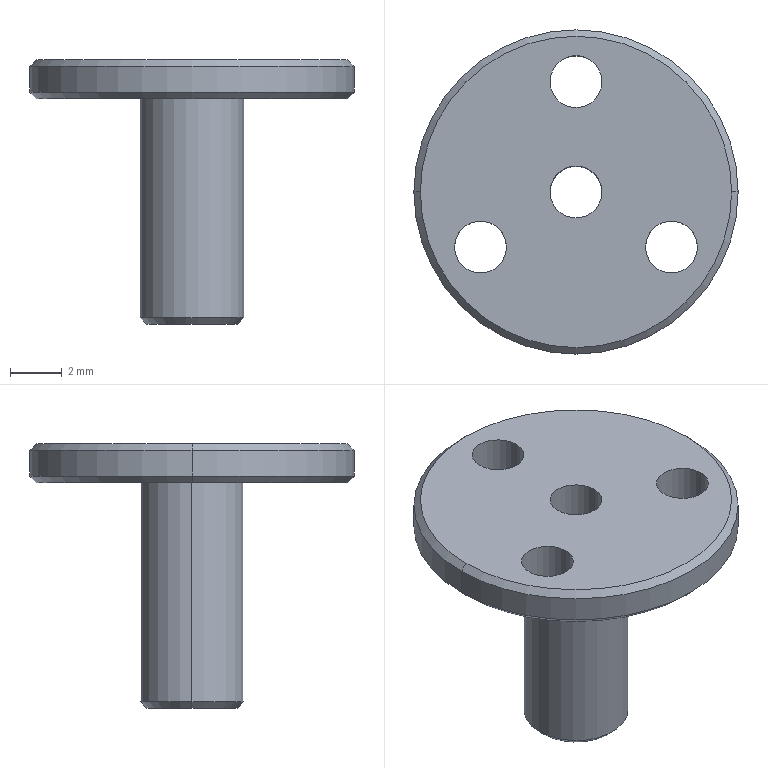Part | NX | features BREP 1 | 1 solid | 21 faces | box 12.5 x 12.5 x 10.2 mm | volume 244.426 mm3 | cylinder 12 | cone 6 | plane 3 | commonest cylinder face diameters 2 x8 4 x2 12.5 x2
STEP:
#1=CARTESIAN_POINT('',(30.496,239.617,-8.7));
#2=VERTEX_POINT('',#1);
#3=CARTESIAN_POINT('',(33.996,239.617,-8.7));
#4=VERTEX_POINT('',#3);
#5=CARTESIAN_POINT('',(32.246,239.617,-8.7));
#6=DIRECTION('',(0.,0.,-1.));
#7=DIRECTION('',(-1.,0.,0.));
#8=AXIS2_PLACEMENT_3D('',#5,#6,#7);
#9=CIRCLE('',#8,1.75);
#10=EDGE_CURVE('',#2,#4,#9,.T.);
#11=ORIENTED_EDGE('',*,*,#10,.F.);
#12=CARTESIAN_POINT('',(30.246,239.617,-8.45));
#13=VERTEX_POINT('',#12);
#14=CARTESIAN_POINT('',(30.496,239.617,-8.7));
#15=DIRECTION('',(-0.7071,0.,0.7071));
#16=VECTOR('',#15,1000.);
#17=LINE('',#14,#16);
#18=EDGE_CURVE('',#2,#13,#17,.T.);
#19=ORIENTED_EDGE('',*,*,#18,.T.);
#20=CARTESIAN_POINT('',(34.246,239.617,-8.45));
#21=VERTEX_POINT('',#20);
#22=CARTESIAN_POINT('',(32.246,239.617,-8.45));
#23=DIRECTION('',(0.,0.,1.));
#24=DIRECTION('',(-1.,0.,0.));
#25=AXIS2_PLACEMENT_3D('',#22,#23,#24);
#26=CIRCLE('',#25,2.);
#27=EDGE_CURVE('',#21,#13,#26,.T.);
#28=ORIENTED_EDGE('',*,*,#27,.F.);
#29=CARTESIAN_POINT('',(33.996,239.617,-8.7));
#30=DIRECTION('',(0.7071,0.,0.7071));
#31=VECTOR('',#30,1000.);
#32=LINE('',#29,#31);
#33=EDGE_CURVE('',#4,#21,#32,.T.);
#34=ORIENTED_EDGE('',*,*,#33,.F.);
#35=EDGE_LOOP('',(#11,#19,#28,#34));
#36=FACE_BOUND('',#35,.T.);
#37=CARTESIAN_POINT('',(32.246,239.617,-8.7));
#38=DIRECTION('',(0.,0.,1.));
#39=DIRECTION('',(-1.,0.,0.));
#40=AXIS2_PLACEMENT_3D('',#37,#38,#39);
#41=CONICAL_SURFACE('',#40,1.75,0.7854);
#42=ADVANCED_FACE('',(#36),#41,.T.);
#43=CARTESIAN_POINT('',(38.246,239.617,1.5));
#44=VERTEX_POINT('',#43);
#45=CARTESIAN_POINT('',(26.246,239.617,1.5));
#46=VERTEX_POINT('',#45);
#47=CARTESIAN_POINT('',(32.246,239.617,1.5));
#48=DIRECTION('',(0.,0.,1.));
#49=DIRECTION('',(1.,0.,0.));
#50=AXIS2_PLACEMENT_3D('',#47,#48,#49);
#51=CIRCLE('',#50,6.);
#52=EDGE_CURVE('',#44,#46,#51,.T.);
#53=ORIENTED_EDGE('',*,*,#52,.F.);
#54=CARTESIAN_POINT('',(38.496,239.617,1.25));
#55=VERTEX_POINT('',#54);
#56=CARTESIAN_POINT('',(38.246,239.617,1.5));
#57=DIRECTION('',(0.7071,0.,-0.7071));
#58=VECTOR('',#57,1000.);
#59=LINE('',#56,#58);
#60=EDGE_CURVE('',#55,#44,#59,.F.);
#61=ORIENTED_EDGE('',*,*,#60,.F.);
#62=CARTESIAN_POINT('',(25.996,239.617,1.25));
#63=VERTEX_POINT('',#62);
#64=CARTESIAN_POINT('',(32.246,239.617,1.25));
#65=DIRECTION('',(0.,0.,-1.));
#66=DIRECTION('',(1.,0.,0.));
#67=AXIS2_PLACEMENT_3D('',#64,#65,#66);
#68=CIRCLE('',#67,6.25);
#69=EDGE_CURVE('',#63,#55,#68,.T.);
#70=ORIENTED_EDGE('',*,*,#69,.F.);
#71=CARTESIAN_POINT('',(26.246,239.617,1.5));
#72=DIRECTION('',(-0.7071,0.,-0.7071));
#73=VECTOR('',#72,1000.);
#74=LINE('',#71,#73);
#75=EDGE_CURVE('',#63,#46,#74,.F.);
#76=ORIENTED_EDGE('',*,*,#75,.T.);
#77=EDGE_LOOP('',(#53,#61,#70,#76));
#78=FACE_BOUND('',#77,.T.);
#79=CARTESIAN_POINT('',(32.246,239.617,1.5));
#80=DIRECTION('',(0.,0.,-1.));
#81=DIRECTION('',(1.,0.,0.));
#82=AXIS2_PLACEMENT_3D('',#79,#80,#81);
#83=CONICAL_SURFACE('',#82,6.,0.7854);
#84=ADVANCED_FACE('',(#78),#83,.T.);
#85=CARTESIAN_POINT('',(26.246,239.617,0.));
#86=VERTEX_POINT('',#85);
#87=CARTESIAN_POINT('',(38.246,239.617,0.));
#88=VERTEX_POINT('',#87);
#89=CARTESIAN_POINT('',(32.246,239.617,0.));
#90=DIRECTION('',(0.,0.,-1.));
#91=DIRECTION('',(1.,0.,0.));
#92=AXIS2_PLACEMENT_3D('',#89,#90,#91);
#93=CIRCLE('',#92,6.);
#94=EDGE_CURVE('',#86,#88,#93,.T.);
#95=ORIENTED_EDGE('',*,*,#94,.F.);
#96=CARTESIAN_POINT('',(25.996,239.617,0.25));
#97=VERTEX_POINT('',#96);
#98=CARTESIAN_POINT('',(25.996,239.617,0.25));
#99=DIRECTION('',(-0.7071,0.,0.7071));
#100=VECTOR('',#99,1000.);
#101=LINE('',#98,#100);
#102=EDGE_CURVE('',#86,#97,#101,.T.);
#103=ORIENTED_EDGE('',*,*,#102,.T.);
#104=CARTESIAN_POINT('',(38.496,239.617,0.25));
#105=VERTEX_POINT('',#104);
#106=CARTESIAN_POINT('',(32.246,239.617,0.25));
#107=DIRECTION('',(0.,0.,1.));
#108=DIRECTION('',(1.,0.,0.));
#109=AXIS2_PLACEMENT_3D('',#106,#107,#108);
#110=CIRCLE('',#109,6.25);
#111=EDGE_CURVE('',#105,#97,#110,.T.);
#112=ORIENTED_EDGE('',*,*,#111,.F.);
#113=CARTESIAN_POINT('',(38.496,239.617,0.25));
#114=DIRECTION('',(0.7071,0.,0.7071));
#115=VECTOR('',#114,1000.);
#116=LINE('',#113,#115);
#117=EDGE_CURVE('',#88,#105,#116,.T.);
#118=ORIENTED_EDGE('',*,*,#117,.F.);
#119=EDGE_LOOP('',(#95,#103,#112,#118));
#120=FACE_BOUND('',#119,.T.);
#121=CARTESIAN_POINT('',(32.246,239.617,0.25));
#122=DIRECTION('',(0.,0.,1.));
#123=DIRECTION('',(-1.,0.,0.));
#124=AXIS2_PLACEMENT_3D('',#121,#122,#123);
#125=CONICAL_SURFACE('',#124,6.25,0.7854);
#126=ADVANCED_FACE('',(#120),#125,.T.);
#127=CARTESIAN_POINT('',(31.246,239.617,1.5));
#128=VERTEX_POINT('',#127);
#129=CARTESIAN_POINT('',(33.246,239.617,1.5));
#130=VERTEX_POINT('',#129);
#131=CARTESIAN_POINT('',(32.246,239.617,1.5));
#132=DIRECTION('',(0.,0.,1.));
#133=DIRECTION('',(1.,0.,0.));
#134=AXIS2_PLACEMENT_3D('',#131,#132,#133);
#135=CIRCLE('',#134,1.);
#136=EDGE_CURVE('',#128,#130,#135,.T.);
#137=ORIENTED_EDGE('',*,*,#136,.T.);
#138=CARTESIAN_POINT('',(33.246,239.617,-8.7));
#139=VERTEX_POINT('',#138);
#140=CARTESIAN_POINT('',(33.246,239.617,-2.7));
#141=DIRECTION('',(0.,0.,-1.));
#142=VECTOR('',#141,1000.);
#143=LINE('',#140,#142);
#144=EDGE_CURVE('',#139,#130,#143,.F.);
#145=ORIENTED_EDGE('',*,*,#144,.F.);
#146=CARTESIAN_POINT('',(31.246,239.617,-8.7));
#147=VERTEX_POINT('',#146);
#148=CARTESIAN_POINT('',(32.246,239.617,-8.7));
#149=DIRECTION('',(0.,0.,-1.));
#150=DIRECTION('',(-1.,0.,0.));
#151=AXIS2_PLACEMENT_3D('',#148,#149,#150);
#152=CIRCLE('',#151,1.);
#153=EDGE_CURVE('',#139,#147,#152,.T.);
#154=ORIENTED_EDGE('',*,*,#153,.T.);
#155=CARTESIAN_POINT('',(31.246,239.617,-2.7));
#156=DIRECTION('',(0.,0.,-1.));
#157=VECTOR('',#156,1000.);
#158=LINE('',#155,#157);
#159=EDGE_CURVE('',#147,#128,#158,.F.);
#160=ORIENTED_EDGE('',*,*,#159,.T.);
#161=EDGE_LOOP('',(#137,#145,#154,#160));
#162=FACE_BOUND('',#161,.T.);
#163=CARTESIAN_POINT('',(32.246,239.617,-2.7));
#164=DIRECTION('',(0.,0.,-1.));
#165=DIRECTION('',(1.,0.,0.));
#166=AXIS2_PLACEMENT_3D('',#163,#164,#165);
#167=CYLINDRICAL_SURFACE('',#166,1.);
#168=ADVANCED_FACE('',(#162),#167,.F.);
#169=ORIENTED_EDGE('',*,*,#27,.T.);
#170=CARTESIAN_POINT('',(30.246,239.617,0.));
#171=VERTEX_POINT('',#170);
#172=CARTESIAN_POINT('',(30.246,239.617,-14.357));
#173=DIRECTION('',(0.,0.,1.));
#174=VECTOR('',#173,1000.);
#175=LINE('',#172,#174);
#176=EDGE_CURVE('',#13,#171,#175,.T.);
#177=ORIENTED_EDGE('',*,*,#176,.T.);
#178=CARTESIAN_POINT('',(34.246,239.617,0.));
#179=VERTEX_POINT('',#178);
#180=CARTESIAN_POINT('',(32.246,239.617,0.));
#181=DIRECTION('',(0.,0.,-1.));
#182=DIRECTION('',(1.,0.,0.));
#183=AXIS2_PLACEMENT_3D('',#180,#181,#182);
#184=CIRCLE('',#183,2.);
#185=EDGE_CURVE('',#171,#179,#184,.T.);
#186=ORIENTED_EDGE('',*,*,#185,.T.);
#187=CARTESIAN_POINT('',(34.246,239.617,-14.357));
#188=DIRECTION('',(0.,0.,1.));
#189=VECTOR('',#188,1000.);
#190=LINE('',#187,#189);
#191=EDGE_CURVE('',#21,#179,#190,.T.);
#192=ORIENTED_EDGE('',*,*,#191,.F.);
#193=EDGE_LOOP('',(#169,#177,#186,#192));
#194=FACE_BOUND('',#193,.T.);
#195=CARTESIAN_POINT('',(32.246,239.617,-14.357));
#196=DIRECTION('',(0.,0.,1.));
#197=DIRECTION('',(-1.,0.,0.));
#198=AXIS2_PLACEMENT_3D('',#195,#196,#197);
#199=CYLINDRICAL_SURFACE('',#198,2.);
#200=ADVANCED_FACE('',(#194),#199,.T.);
#201=CARTESIAN_POINT('',(27.566,237.492,1.5));
#202=VERTEX_POINT('',#201);
#203=CARTESIAN_POINT('',(29.566,237.492,1.5));
#204=VERTEX_POINT('',#203);
#205=CARTESIAN_POINT('',(28.566,237.492,1.5));
#206=DIRECTION('',(0.,0.,1.));
#207=DIRECTION('',(1.,0.,0.));
#208=AXIS2_PLACEMENT_3D('',#205,#206,#207);
#209=CIRCLE('',#208,1.);
#210=EDGE_CURVE('',#202,#204,#209,.T.);
#211=ORIENTED_EDGE('',*,*,#210,.T.);
#212=CARTESIAN_POINT('',(29.566,237.492,0.));
#213=VERTEX_POINT('',#212);
#214=CARTESIAN_POINT('',(29.566,237.492,1.5));
#215=DIRECTION('',(0.,0.,-1.));
#216=VECTOR('',#215,1000.);
#217=LINE('',#214,#216);
#218=EDGE_CURVE('',#213,#204,#217,.F.);
#219=ORIENTED_EDGE('',*,*,#218,.F.);
#220=CARTESIAN_POINT('',(27.566,237.492,0.));
#221=VERTEX_POINT('',#220);
#222=CARTESIAN_POINT('',(28.566,237.492,0.));
#223=DIRECTION('',(0.,0.,1.));
#224=DIRECTION('',(1.,0.,0.));
#225=AXIS2_PLACEMENT_3D('',#222,#223,#224);
#226=CIRCLE('',#225,1.);
#227=EDGE_CURVE('',#221,#213,#226,.T.);
#228=ORIENTED_EDGE('',*,*,#227,.F.);
#229=CARTESIAN_POINT('',(27.566,237.492,1.5));
#230=DIRECTION('',(0.,0.,-1.));
#231=VECTOR('',#230,1000.);
#232=LINE('',#229,#231);
#233=EDGE_CURVE('',#221,#202,#232,.F.);
#234=ORIENTED_EDGE('',*,*,#233,.T.);
#235=EDGE_LOOP('',(#211,#219,#228,#234));
#236=FACE_BOUND('',#235,.T.);
#237=CARTESIAN_POINT('',(28.566,237.492,1.5));
#238=DIRECTION('',(0.,0.,-1.));
#239=DIRECTION('',(1.,0.,0.));
#240=AXIS2_PLACEMENT_3D('',#237,#238,#239);
#241=CYLINDRICAL_SURFACE('',#240,1.);
#242=ADVANCED_FACE('',(#236),#241,.F.);
#243=CARTESIAN_POINT('',(34.927,237.492,1.5));
#244=VERTEX_POINT('',#243);
#245=CARTESIAN_POINT('',(36.927,237.492,1.5));
#246=VERTEX_POINT('',#245);
#247=CARTESIAN_POINT('',(35.927,237.492,1.5));
#248=DIRECTION('',(0.,0.,1.));
#249=DIRECTION('',(1.,0.,0.));
#250=AXIS2_PLACEMENT_3D('',#247,#248,#249);
#251=CIRCLE('',#250,1.);
#252=EDGE_CURVE('',#244,#246,#251,.T.);
#253=ORIENTED_EDGE('',*,*,#252,.T.);
#254=CARTESIAN_POINT('',(36.927,237.492,0.));
#255=VERTEX_POINT('',#254);
#256=CARTESIAN_POINT('',(36.927,237.492,1.5));
#257=DIRECTION('',(0.,0.,-1.));
#258=VECTOR('',#257,1000.);
#259=LINE('',#256,#258);
#260=EDGE_CURVE('',#255,#246,#259,.F.);
#261=ORIENTED_EDGE('',*,*,#260,.F.);
#262=CARTESIAN_POINT('',(34.927,237.492,0.));
#263=VERTEX_POINT('',#262);
#264=CARTESIAN_POINT('',(35.927,237.492,0.));
#265=DIRECTION('',(0.,0.,1.));
#266=DIRECTION('',(1.,0.,0.));
#267=AXIS2_PLACEMENT_3D('',#264,#265,#266);
#268=CIRCLE('',#267,1.);
#269=EDGE_CURVE('',#263,#255,#268,.T.);
#270=ORIENTED_EDGE('',*,*,#269,.F.);
#271=CARTESIAN_POINT('',(34.927,237.492,1.5));
#272=DIRECTION('',(0.,0.,-1.));
#273=VECTOR('',#272,1000.);
#274=LINE('',#271,#273);
#275=EDGE_CURVE('',#263,#244,#274,.F.);
#276=ORIENTED_EDGE('',*,*,#275,.T.);
#277=EDGE_LOOP('',(#253,#261,#270,#276));
#278=FACE_BOUND('',#277,.T.);
#279=CARTESIAN_POINT('',(35.927,237.492,1.5));
#280=DIRECTION('',(0.,0.,-1.));
#281=DIRECTION('',(1.,0.,0.));
#282=AXIS2_PLACEMENT_3D('',#279,#280,#281);
#283=CYLINDRICAL_SURFACE('',#282,1.);
#284=ADVANCED_FACE('',(#278),#283,.F.);
#285=CARTESIAN_POINT('',(31.246,243.867,1.5));
#286=VERTEX_POINT('',#285);
#287=CARTESIAN_POINT('',(33.246,243.867,1.5));
#288=VERTEX_POINT('',#287);
#289=CARTESIAN_POINT('',(32.246,243.867,1.5));
#290=DIRECTION('',(0.,0.,1.));
#291=DIRECTION('',(1.,0.,0.));
#292=AXIS2_PLACEMENT_3D('',#289,#290,#291);
#293=CIRCLE('',#292,1.);
#294=EDGE_CURVE('',#286,#288,#293,.T.);
#295=ORIENTED_EDGE('',*,*,#294,.T.);
#296=CARTESIAN_POINT('',(33.246,243.867,0.));
#297=VERTEX_POINT('',#296);
#298=CARTESIAN_POINT('',(33.246,243.867,1.5));
#299=DIRECTION('',(0.,0.,-1.));
#300=VECTOR('',#299,1000.);
#301=LINE('',#298,#300);
#302=EDGE_CURVE('',#297,#288,#301,.F.);
#303=ORIENTED_EDGE('',*,*,#302,.F.);
#304=CARTESIAN_POINT('',(31.246,243.867,0.));
#305=VERTEX_POINT('',#304);
#306=CARTESIAN_POINT('',(32.246,243.867,0.));
#307=DIRECTION('',(0.,0.,1.));
#308=DIRECTION('',(1.,0.,0.));
#309=AXIS2_PLACEMENT_3D('',#306,#307,#308);
#310=CIRCLE('',#309,1.);
#311=EDGE_CURVE('',#305,#297,#310,.T.);
#312=ORIENTED_EDGE('',*,*,#311,.F.);
#313=CARTESIAN_POINT('',(31.246,243.867,1.5));
#314=DIRECTION('',(0.,0.,-1.));
#315=VECTOR('',#314,1000.);
#316=LINE('',#313,#315);
#317=EDGE_CURVE('',#305,#286,#316,.F.);
#318=ORIENTED_EDGE('',*,*,#317,.T.);
#319=EDGE_LOOP('',(#295,#303,#312,#318));
#320=FACE_BOUND('',#319,.T.);
#321=CARTESIAN_POINT('',(32.246,243.867,1.5));
#322=DIRECTION('',(0.,0.,-1.));
#323=DIRECTION('',(1.,0.,0.));
#324=AXIS2_PLACEMENT_3D('',#321,#322,#323);
#325=CYLINDRICAL_SURFACE('',#324,1.);
#326=ADVANCED_FACE('',(#320),#325,.F.);
#327=ORIENTED_EDGE('',*,*,#69,.T.);
#328=CARTESIAN_POINT('',(38.496,239.617,1.5));
#329=DIRECTION('',(0.,0.,-1.));
#330=VECTOR('',#329,1000.);
#331=LINE('',#328,#330);
#332=EDGE_CURVE('',#105,#55,#331,.F.);
#333=ORIENTED_EDGE('',*,*,#332,.F.);
#334=ORIENTED_EDGE('',*,*,#111,.T.);
#335=CARTESIAN_POINT('',(25.996,239.617,1.5));
#336=DIRECTION('',(0.,0.,-1.));
#337=VECTOR('',#336,1000.);
#338=LINE('',#335,#337);
#339=EDGE_CURVE('',#97,#63,#338,.F.);
#340=ORIENTED_EDGE('',*,*,#339,.T.);
#341=EDGE_LOOP('',(#327,#333,#334,#340));
#342=FACE_BOUND('',#341,.T.);
#343=CARTESIAN_POINT('',(32.246,239.617,1.5));
#344=DIRECTION('',(0.,0.,-1.));
#345=DIRECTION('',(1.,0.,0.));
#346=AXIS2_PLACEMENT_3D('',#343,#344,#345);
#347=CYLINDRICAL_SURFACE('',#346,6.25);
#348=ADVANCED_FACE('',(#342),#347,.T.);
#349=CARTESIAN_POINT('',(32.246,239.617,1.5));
#350=DIRECTION('',(0.,0.,1.));
#351=DIRECTION('',(1.,0.,0.));
#352=AXIS2_PLACEMENT_3D('',#349,#350,#351);
#353=CIRCLE('',#352,6.);
#354=EDGE_CURVE('',#46,#44,#353,.T.);
#355=ORIENTED_EDGE('',*,*,#354,.T.);
#356=ORIENTED_EDGE('',*,*,#52,.T.);
#357=EDGE_LOOP('',(#355,#356));
#358=FACE_BOUND('',#357,.T.);
#359=ORIENTED_EDGE('',*,*,#136,.F.);
#360=CARTESIAN_POINT('',(32.246,239.617,1.5));
#361=DIRECTION('',(0.,0.,1.));
#362=DIRECTION('',(1.,0.,0.));
#363=AXIS2_PLACEMENT_3D('',#360,#361,#362);
#364=CIRCLE('',#363,1.);
#365=EDGE_CURVE('',#130,#128,#364,.T.);
#366=ORIENTED_EDGE('',*,*,#365,.F.);
#367=EDGE_LOOP('',(#359,#366));
#368=FACE_BOUND('',#367,.T.);
#369=ORIENTED_EDGE('',*,*,#252,.F.);
#370=CARTESIAN_POINT('',(35.927,237.492,1.5));
#371=DIRECTION('',(0.,0.,1.));
#372=DIRECTION('',(1.,0.,0.));
#373=AXIS2_PLACEMENT_3D('',#370,#371,#372);
#374=CIRCLE('',#373,1.);
#375=EDGE_CURVE('',#246,#244,#374,.T.);
#376=ORIENTED_EDGE('',*,*,#375,.F.);
#377=EDGE_LOOP('',(#369,#376));
#378=FACE_BOUND('',#377,.T.);
#379=ORIENTED_EDGE('',*,*,#294,.F.);
#380=CARTESIAN_POINT('',(32.246,243.867,1.5));
#381=DIRECTION('',(0.,0.,1.));
#382=DIRECTION('',(1.,0.,0.));
#383=AXIS2_PLACEMENT_3D('',#380,#381,#382);
#384=CIRCLE('',#383,1.);
#385=EDGE_CURVE('',#288,#286,#384,.T.);
#386=ORIENTED_EDGE('',*,*,#385,.F.);
#387=EDGE_LOOP('',(#379,#386));
#388=FACE_BOUND('',#387,.T.);
#389=ORIENTED_EDGE('',*,*,#210,.F.);
#390=CARTESIAN_POINT('',(28.566,237.492,1.5));
#391=DIRECTION('',(0.,0.,1.));
#392=DIRECTION('',(1.,0.,0.));
#393=AXIS2_PLACEMENT_3D('',#390,#391,#392);
#394=CIRCLE('',#393,1.);
#395=EDGE_CURVE('',#204,#202,#394,.T.);
#396=ORIENTED_EDGE('',*,*,#395,.F.);
#397=EDGE_LOOP('',(#389,#396));
#398=FACE_BOUND('',#397,.T.);
#399=CARTESIAN_POINT('',(32.246,239.617,1.5));
#400=DIRECTION('',(0.,0.,1.));
#401=DIRECTION('',(-1.,0.,0.));
#402=AXIS2_PLACEMENT_3D('',#399,#400,#401);
#403=PLANE('',#402);
#404=ADVANCED_FACE('',(#358,#368,#378,#388,#398),#403,.T.);
#405=CARTESIAN_POINT('',(32.246,239.617,0.));
#406=DIRECTION('',(0.,0.,-1.));
#407=DIRECTION('',(1.,0.,0.));
#408=AXIS2_PLACEMENT_3D('',#405,#406,#407);
#409=CIRCLE('',#408,6.);
#410=EDGE_CURVE('',#88,#86,#409,.T.);
#411=ORIENTED_EDGE('',*,*,#410,.T.);
#412=ORIENTED_EDGE('',*,*,#94,.T.);
#413=EDGE_LOOP('',(#411,#412));
#414=FACE_BOUND('',#413,.T.);
#415=CARTESIAN_POINT('',(32.246,239.617,0.));
#416=DIRECTION('',(0.,0.,-1.));
#417=DIRECTION('',(1.,0.,0.));
#418=AXIS2_PLACEMENT_3D('',#415,#416,#417);
#419=CIRCLE('',#418,2.);
#420=EDGE_CURVE('',#179,#171,#419,.T.);
#421=ORIENTED_EDGE('',*,*,#420,.F.);
#422=ORIENTED_EDGE('',*,*,#185,.F.);
#423=EDGE_LOOP('',(#421,#422));
#424=FACE_BOUND('',#423,.T.);
#425=ORIENTED_EDGE('',*,*,#311,.T.);
#426=CARTESIAN_POINT('',(32.246,243.867,0.));
#427=DIRECTION('',(0.,0.,1.));
#428=DIRECTION('',(1.,0.,0.));
#429=AXIS2_PLACEMENT_3D('',#426,#427,#428);
#430=CIRCLE('',#429,1.);
#431=EDGE_CURVE('',#297,#305,#430,.T.);
#432=ORIENTED_EDGE('',*,*,#431,.T.);
#433=EDGE_LOOP('',(#425,#432));
#434=FACE_BOUND('',#433,.T.);
#435=ORIENTED_EDGE('',*,*,#269,.T.);
#436=CARTESIAN_POINT('',(35.927,237.492,0.));
#437=DIRECTION('',(0.,0.,1.));
#438=DIRECTION('',(1.,0.,0.));
#439=AXIS2_PLACEMENT_3D('',#436,#437,#438);
#440=CIRCLE('',#439,1.);
#441=EDGE_CURVE('',#255,#263,#440,.T.);
#442=ORIENTED_EDGE('',*,*,#441,.T.);
#443=EDGE_LOOP('',(#435,#442));
#444=FACE_BOUND('',#443,.T.);
#445=ORIENTED_EDGE('',*,*,#227,.T.);
#446=CARTESIAN_POINT('',(28.566,237.492,0.));
#447=DIRECTION('',(0.,0.,1.));
#448=DIRECTION('',(1.,0.,0.));
#449=AXIS2_PLACEMENT_3D('',#446,#447,#448);
#450=CIRCLE('',#449,1.);
#451=EDGE_CURVE('',#213,#221,#450,.T.);
#452=ORIENTED_EDGE('',*,*,#451,.T.);
#453=EDGE_LOOP('',(#445,#452));
#454=FACE_BOUND('',#453,.T.);
#455=CARTESIAN_POINT('',(32.246,239.617,0.));
#456=DIRECTION('',(0.,0.,1.));
#457=DIRECTION('',(-1.,0.,0.));
#458=AXIS2_PLACEMENT_3D('',#455,#456,#457);
#459=PLANE('',#458);
#460=ADVANCED_FACE('',(#414,#424,#434,#444,#454),#459,.F.);
#461=ORIENTED_EDGE('',*,*,#332,.T.);
#462=CARTESIAN_POINT('',(32.246,239.617,1.25));
#463=DIRECTION('',(0.,0.,-1.));
#464=DIRECTION('',(1.,0.,0.));
#465=AXIS2_PLACEMENT_3D('',#462,#463,#464);
#466=CIRCLE('',#465,6.25);
#467=EDGE_CURVE('',#55,#63,#466,.T.);
#468=ORIENTED_EDGE('',*,*,#467,.T.);
#469=ORIENTED_EDGE('',*,*,#339,.F.);
#470=CARTESIAN_POINT('',(32.246,239.617,0.25));
#471=DIRECTION('',(0.,0.,1.));
#472=DIRECTION('',(1.,0.,0.));
#473=AXIS2_PLACEMENT_3D('',#470,#471,#472);
#474=CIRCLE('',#473,6.25);
#475=EDGE_CURVE('',#97,#105,#474,.T.);
#476=ORIENTED_EDGE('',*,*,#475,.T.);
#477=EDGE_LOOP('',(#461,#468,#469,#476));
#478=FACE_BOUND('',#477,.T.);
#479=CARTESIAN_POINT('',(32.246,239.617,1.5));
#480=DIRECTION('',(0.,0.,-1.));
#481=DIRECTION('',(1.,0.,0.));
#482=AXIS2_PLACEMENT_3D('',#479,#480,#481);
#483=CYLINDRICAL_SURFACE('',#482,6.25);
#484=ADVANCED_FACE('',(#478),#483,.T.);
#485=ORIENTED_EDGE('',*,*,#302,.T.);
#486=ORIENTED_EDGE('',*,*,#385,.T.);
#487=ORIENTED_EDGE('',*,*,#317,.F.);
#488=ORIENTED_EDGE('',*,*,#431,.F.);
#489=EDGE_LOOP('',(#485,#486,#487,#488));
#490=FACE_BOUND('',#489,.T.);
#491=CARTESIAN_POINT('',(32.246,243.867,1.5));
#492=DIRECTION('',(0.,0.,-1.));
#493=DIRECTION('',(1.,0.,0.));
#494=AXIS2_PLACEMENT_3D('',#491,#492,#493);
#495=CYLINDRICAL_SURFACE('',#494,1.);
#496=ADVANCED_FACE('',(#490),#495,.F.);
#497=ORIENTED_EDGE('',*,*,#260,.T.);
#498=ORIENTED_EDGE('',*,*,#375,.T.);
#499=ORIENTED_EDGE('',*,*,#275,.F.);
#500=ORIENTED_EDGE('',*,*,#441,.F.);
#501=EDGE_LOOP('',(#497,#498,#499,#500));
#502=FACE_BOUND('',#501,.T.);
#503=CARTESIAN_POINT('',(35.927,237.492,1.5));
#504=DIRECTION('',(0.,0.,-1.));
#505=DIRECTION('',(1.,0.,0.));
#506=AXIS2_PLACEMENT_3D('',#503,#504,#505);
#507=CYLINDRICAL_SURFACE('',#506,1.);
#508=ADVANCED_FACE('',(#502),#507,.F.);
#509=ORIENTED_EDGE('',*,*,#218,.T.);
#510=ORIENTED_EDGE('',*,*,#395,.T.);
#511=ORIENTED_EDGE('',*,*,#233,.F.);
#512=ORIENTED_EDGE('',*,*,#451,.F.);
#513=EDGE_LOOP('',(#509,#510,#511,#512));
#514=FACE_BOUND('',#513,.T.);
#515=CARTESIAN_POINT('',(28.566,237.492,1.5));
#516=DIRECTION('',(0.,0.,-1.));
#517=DIRECTION('',(1.,0.,0.));
#518=AXIS2_PLACEMENT_3D('',#515,#516,#517);
#519=CYLINDRICAL_SURFACE('',#518,1.);
#520=ADVANCED_FACE('',(#514),#519,.F.);
#521=ORIENTED_EDGE('',*,*,#176,.F.);
#522=CARTESIAN_POINT('',(32.246,239.617,-8.45));
#523=DIRECTION('',(0.,0.,1.));
#524=DIRECTION('',(-1.,0.,0.));
#525=AXIS2_PLACEMENT_3D('',#522,#523,#524);
#526=CIRCLE('',#525,2.);
#527=EDGE_CURVE('',#13,#21,#526,.T.);
#528=ORIENTED_EDGE('',*,*,#527,.T.);
#529=ORIENTED_EDGE('',*,*,#191,.T.);
#530=ORIENTED_EDGE('',*,*,#420,.T.);
#531=EDGE_LOOP('',(#521,#528,#529,#530));
#532=FACE_BOUND('',#531,.T.);
#533=CARTESIAN_POINT('',(32.246,239.617,-14.357));
#534=DIRECTION('',(0.,0.,1.));
#535=DIRECTION('',(-1.,0.,0.));
#536=AXIS2_PLACEMENT_3D('',#533,#534,#535);
#537=CYLINDRICAL_SURFACE('',#536,2.);
#538=ADVANCED_FACE('',(#532),#537,.T.);
#539=CARTESIAN_POINT('',(32.246,239.617,-8.7));
#540=DIRECTION('',(0.,0.,-1.));
#541=DIRECTION('',(-1.,0.,0.));
#542=AXIS2_PLACEMENT_3D('',#539,#540,#541);
#543=CIRCLE('',#542,1.75);
#544=EDGE_CURVE('',#4,#2,#543,.T.);
#545=ORIENTED_EDGE('',*,*,#544,.T.);
#546=ORIENTED_EDGE('',*,*,#10,.T.);
#547=EDGE_LOOP('',(#545,#546));
#548=FACE_BOUND('',#547,.T.);
#549=CARTESIAN_POINT('',(32.246,239.617,-8.7));
#550=DIRECTION('',(0.,0.,-1.));
#551=DIRECTION('',(-1.,0.,0.));
#552=AXIS2_PLACEMENT_3D('',#549,#550,#551);
#553=CIRCLE('',#552,1.);
#554=EDGE_CURVE('',#147,#139,#553,.T.);
#555=ORIENTED_EDGE('',*,*,#554,.F.);
#556=ORIENTED_EDGE('',*,*,#153,.F.);
#557=EDGE_LOOP('',(#555,#556));
#558=FACE_BOUND('',#557,.T.);
#559=CARTESIAN_POINT('',(29.103,240.218,-8.7));
#560=DIRECTION('',(0.,0.,-1.));
#561=DIRECTION('',(0.,1.,0.));
#562=AXIS2_PLACEMENT_3D('',#559,#560,#561);
#563=PLANE('',#562);
#564=ADVANCED_FACE('',(#548,#558),#563,.T.);
#565=ORIENTED_EDGE('',*,*,#144,.T.);
#566=ORIENTED_EDGE('',*,*,#365,.T.);
#567=ORIENTED_EDGE('',*,*,#159,.F.);
#568=ORIENTED_EDGE('',*,*,#554,.T.);
#569=EDGE_LOOP('',(#565,#566,#567,#568));
#570=FACE_BOUND('',#569,.T.);
#571=CARTESIAN_POINT('',(32.246,239.617,-2.7));
#572=DIRECTION('',(0.,0.,-1.));
#573=DIRECTION('',(1.,0.,0.));
#574=AXIS2_PLACEMENT_3D('',#571,#572,#573);
#575=CYLINDRICAL_SURFACE('',#574,1.);
#576=ADVANCED_FACE('',(#570),#575,.F.);
#577=ORIENTED_EDGE('',*,*,#102,.F.);
#578=ORIENTED_EDGE('',*,*,#410,.F.);
#579=ORIENTED_EDGE('',*,*,#117,.T.);
#580=ORIENTED_EDGE('',*,*,#475,.F.);
#581=EDGE_LOOP('',(#577,#578,#579,#580));
#582=FACE_BOUND('',#581,.T.);
#583=CARTESIAN_POINT('',(32.246,239.617,0.25));
#584=DIRECTION('',(0.,0.,1.));
#585=DIRECTION('',(-1.,0.,0.));
#586=AXIS2_PLACEMENT_3D('',#583,#584,#585);
#587=CONICAL_SURFACE('',#586,6.25,0.7854);
#588=ADVANCED_FACE('',(#582),#587,.T.);
#589=ORIENTED_EDGE('',*,*,#60,.T.);
#590=ORIENTED_EDGE('',*,*,#354,.F.);
#591=ORIENTED_EDGE('',*,*,#75,.F.);
#592=ORIENTED_EDGE('',*,*,#467,.F.);
#593=EDGE_LOOP('',(#589,#590,#591,#592));
#594=FACE_BOUND('',#593,.T.);
#595=CARTESIAN_POINT('',(32.246,239.617,1.5));
#596=DIRECTION('',(0.,0.,-1.));
#597=DIRECTION('',(1.,0.,0.));
#598=AXIS2_PLACEMENT_3D('',#595,#596,#597);
#599=CONICAL_SURFACE('',#598,6.,0.7854);
#600=ADVANCED_FACE('',(#594),#599,.T.);
#601=ORIENTED_EDGE('',*,*,#18,.F.);
#602=ORIENTED_EDGE('',*,*,#544,.F.);
#603=ORIENTED_EDGE('',*,*,#33,.T.);
#604=ORIENTED_EDGE('',*,*,#527,.F.);
#605=EDGE_LOOP('',(#601,#602,#603,#604));
#606=FACE_BOUND('',#605,.T.);
#607=CARTESIAN_POINT('',(32.246,239.617,-8.7));
#608=DIRECTION('',(0.,0.,1.));
#609=DIRECTION('',(-1.,0.,0.));
#610=AXIS2_PLACEMENT_3D('',#607,#608,#609);
#611=CONICAL_SURFACE('',#610,1.75,0.7854);
#612=ADVANCED_FACE('',(#606),#611,.T.);
#613=CLOSED_SHELL('',(#42,#84,#126,#168,#200,#242,#284,#326,#348,#404,#460,#484,#496,#508,#520,#538,#564,#576,#588,#600,#612));
#614=MANIFOLD_SOLID_BREP('',#613);
#615=(LENGTH_UNIT()NAMED_UNIT(*)SI_UNIT(.MILLI.,.METRE.));
#616=UNCERTAINTY_MEASURE_WITH_UNIT(LENGTH_MEASURE(0.00001),#615,'','');
#617=(NAMED_UNIT(*)PLANE_ANGLE_UNIT()SI_UNIT($,.RADIAN.));
#618=(NAMED_UNIT(*)SI_UNIT($,.STERADIAN.)SOLID_ANGLE_UNIT());
#619=(GEOMETRIC_REPRESENTATION_CONTEXT(3)GLOBAL_UNCERTAINTY_ASSIGNED_CONTEXT((#616))GLOBAL_UNIT_ASSIGNED_CONTEXT((#615,#617,#618))REPRESENTATION_CONTEXT('',''));
#620=ADVANCED_BREP_SHAPE_REPRESENTATION('',(#614),#619);